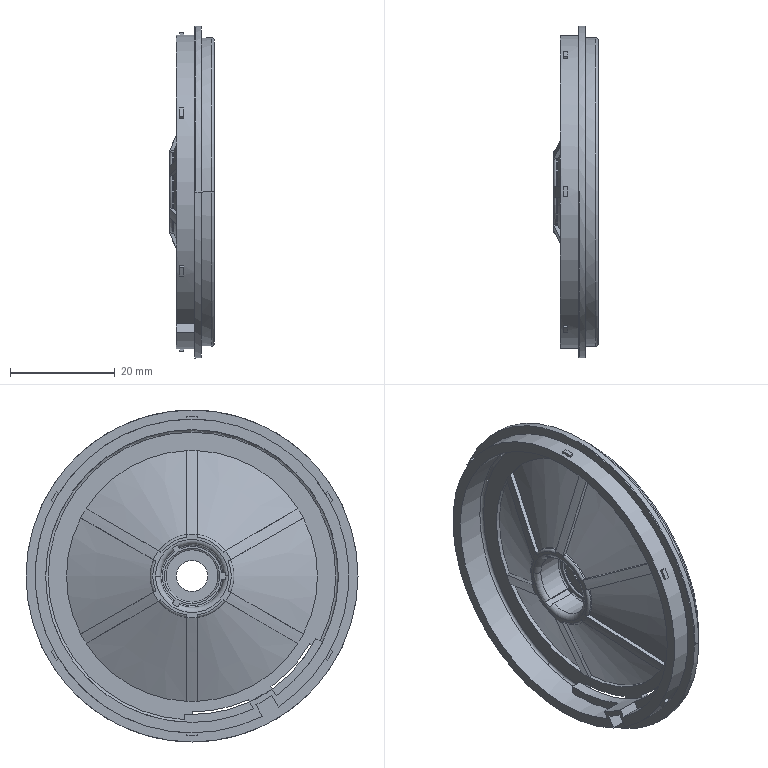Part | STEP file | SHANGAI_7_1 | 1 solid | 139 faces | box 8.5 x 63.5 x 63.5 mm | volume 5943 mm3 | plane 68 | cylinder 39 | torus 18 | cone 14 | commonest cylinder face diameters 16 x8 48 x6 61 x6 12 x3 56 x3 6 x2